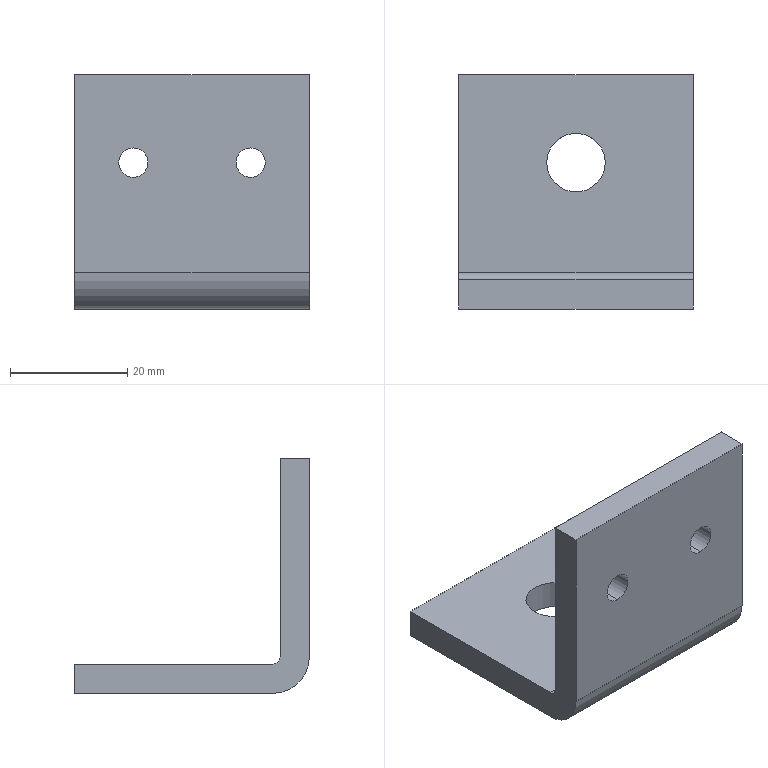Part | SolidWorks | features ICE 2, Extrusion 1 | 1 solid | 16 faces | box 40 x 40 x 40 mm | volume 14089 mm3 | cylinder 8 | plane 8 | commonest cylinder face diameters 5 x4 10 x2 2.5 x1 12.5 x1
STEP:
#1=CARTESIAN_POINT('',(-0.3937,-0.5659,0.421));
#2=VERTEX_POINT('',#1);
#3=CARTESIAN_POINT('',(-0.3937,-0.5659,0.2242));
#4=VERTEX_POINT('',#3);
#5=CARTESIAN_POINT('',(-0.3937,-0.5659,0.3226));
#6=DIRECTION('',(0.,-1.,0.));
#7=DIRECTION('',(0.,0.,-1.));
#8=AXIS2_PLACEMENT_3D('',#5,#6,#7);
#9=CIRCLE('',#8,0.09843);
#10=EDGE_CURVE('',#2,#4,#9,.T.);
#11=ORIENTED_EDGE('',*,*,#10,.T.);
#12=CARTESIAN_POINT('',(-0.3937,-0.3691,0.2242));
#13=VERTEX_POINT('',#12);
#14=CARTESIAN_POINT('',(-0.3937,-1.944,0.2242));
#15=DIRECTION('',(0.,1.,0.));
#16=VECTOR('',#15,39.37);
#17=LINE('',#14,#16);
#18=EDGE_CURVE('',#4,#13,#17,.T.);
#19=ORIENTED_EDGE('',*,*,#18,.T.);
#20=CARTESIAN_POINT('',(-0.3937,-0.3691,0.421));
#21=VERTEX_POINT('',#20);
#22=CARTESIAN_POINT('',(-0.3937,-0.3691,0.3226));
#23=DIRECTION('',(0.,1.,0.));
#24=DIRECTION('',(0.,0.,1.));
#25=AXIS2_PLACEMENT_3D('',#22,#23,#24);
#26=CIRCLE('',#25,0.09843);
#27=EDGE_CURVE('',#13,#21,#26,.T.);
#28=ORIENTED_EDGE('',*,*,#27,.T.);
#29=CARTESIAN_POINT('',(-0.3937,-1.944,0.421));
#30=DIRECTION('',(0.,1.,0.));
#31=VECTOR('',#30,39.37);
#32=LINE('',#29,#31);
#33=EDGE_CURVE('',#2,#21,#32,.T.);
#34=ORIENTED_EDGE('',*,*,#33,.F.);
#35=EDGE_LOOP('',(#11,#19,#28,#34));
#36=FACE_OUTER_BOUND('',#35,.T.);
#37=CARTESIAN_POINT('',(-0.3937,-1.944,0.3226));
#38=DIRECTION('',(0.,1.,0.));
#39=DIRECTION('',(0.,0.,1.));
#40=AXIS2_PLACEMENT_3D('',#37,#38,#39);
#41=CYLINDRICAL_SURFACE('',#40,0.09843);
#42=ADVANCED_FACE('',(#36),#41,.F.);
#43=CARTESIAN_POINT('',(-1.181,-0.5659,0.421));
#44=VERTEX_POINT('',#43);
#45=CARTESIAN_POINT('',(-1.181,-0.5659,0.2242));
#46=VERTEX_POINT('',#45);
#47=CARTESIAN_POINT('',(-1.181,-0.5659,0.3226));
#48=DIRECTION('',(0.,-1.,0.));
#49=DIRECTION('',(0.,0.,-1.));
#50=AXIS2_PLACEMENT_3D('',#47,#48,#49);
#51=CIRCLE('',#50,0.09843);
#52=EDGE_CURVE('',#44,#46,#51,.T.);
#53=ORIENTED_EDGE('',*,*,#52,.T.);
#54=CARTESIAN_POINT('',(-1.181,-0.3691,0.2242));
#55=VERTEX_POINT('',#54);
#56=CARTESIAN_POINT('',(-1.181,-1.944,0.2242));
#57=DIRECTION('',(0.,1.,0.));
#58=VECTOR('',#57,39.37);
#59=LINE('',#56,#58);
#60=EDGE_CURVE('',#46,#55,#59,.T.);
#61=ORIENTED_EDGE('',*,*,#60,.T.);
#62=CARTESIAN_POINT('',(-1.181,-0.3691,0.421));
#63=VERTEX_POINT('',#62);
#64=CARTESIAN_POINT('',(-1.181,-0.3691,0.3226));
#65=DIRECTION('',(0.,1.,0.));
#66=DIRECTION('',(0.,0.,1.));
#67=AXIS2_PLACEMENT_3D('',#64,#65,#66);
#68=CIRCLE('',#67,0.09843);
#69=EDGE_CURVE('',#55,#63,#68,.T.);
#70=ORIENTED_EDGE('',*,*,#69,.T.);
#71=CARTESIAN_POINT('',(-1.181,-1.944,0.421));
#72=DIRECTION('',(0.,1.,0.));
#73=VECTOR('',#72,39.37);
#74=LINE('',#71,#73);
#75=EDGE_CURVE('',#44,#63,#74,.T.);
#76=ORIENTED_EDGE('',*,*,#75,.F.);
#77=EDGE_LOOP('',(#53,#61,#70,#76));
#78=FACE_OUTER_BOUND('',#77,.T.);
#79=CARTESIAN_POINT('',(-1.181,-1.944,0.3226));
#80=DIRECTION('',(0.,1.,0.));
#81=DIRECTION('',(0.,0.,1.));
#82=AXIS2_PLACEMENT_3D('',#79,#80,#81);
#83=CYLINDRICAL_SURFACE('',#82,0.09843);
#84=ADVANCED_FACE('',(#78),#83,.F.);
#85=CARTESIAN_POINT('',(-0.5906,0.4183,-0.6616));
#86=VERTEX_POINT('',#85);
#87=CARTESIAN_POINT('',(-0.9843,0.4183,-0.6616));
#88=VERTEX_POINT('',#87);
#89=CARTESIAN_POINT('',(-0.7874,0.4183,-0.6616));
#90=DIRECTION('',(0.,0.,-1.));
#91=DIRECTION('',(-1.,0.,0.));
#92=AXIS2_PLACEMENT_3D('',#89,#90,#91);
#93=CIRCLE('',#92,0.1969);
#94=EDGE_CURVE('',#86,#88,#93,.T.);
#95=ORIENTED_EDGE('',*,*,#94,.T.);
#96=CARTESIAN_POINT('',(-0.9843,0.4183,-0.4648));
#97=VERTEX_POINT('',#96);
#98=CARTESIAN_POINT('',(-0.9843,0.4183,-2.04));
#99=DIRECTION('',(0.,0.,1.));
#100=VECTOR('',#99,39.37);
#101=LINE('',#98,#100);
#102=EDGE_CURVE('',#88,#97,#101,.T.);
#103=ORIENTED_EDGE('',*,*,#102,.T.);
#104=CARTESIAN_POINT('',(-0.5906,0.4183,-0.4648));
#105=VERTEX_POINT('',#104);
#106=CARTESIAN_POINT('',(-0.7874,0.4183,-0.4648));
#107=DIRECTION('',(0.,0.,1.));
#108=DIRECTION('',(1.,0.,0.));
#109=AXIS2_PLACEMENT_3D('',#106,#107,#108);
#110=CIRCLE('',#109,0.1969);
#111=EDGE_CURVE('',#97,#105,#110,.T.);
#112=ORIENTED_EDGE('',*,*,#111,.T.);
#113=CARTESIAN_POINT('',(-0.5906,0.4183,-2.04));
#114=DIRECTION('',(0.,0.,1.));
#115=VECTOR('',#114,39.37);
#116=LINE('',#113,#115);
#117=EDGE_CURVE('',#86,#105,#116,.T.);
#118=ORIENTED_EDGE('',*,*,#117,.F.);
#119=EDGE_LOOP('',(#95,#103,#112,#118));
#120=FACE_OUTER_BOUND('',#119,.T.);
#121=CARTESIAN_POINT('',(-0.7874,0.4183,-2.04));
#122=DIRECTION('',(0.,0.,1.));
#123=DIRECTION('',(1.,0.,0.));
#124=AXIS2_PLACEMENT_3D('',#121,#122,#123);
#125=CYLINDRICAL_SURFACE('',#124,0.1969);
#126=ADVANCED_FACE('',(#120),#125,.F.);
#127=CARTESIAN_POINT('',(0.,1.009,-0.6616));
#128=VERTEX_POINT('',#127);
#129=CARTESIAN_POINT('',(0.,1.009,-0.4648));
#130=VERTEX_POINT('',#129);
#131=CARTESIAN_POINT('',(0.,1.009,-0.6616));
#132=DIRECTION('',(0.,0.,1.));
#133=VECTOR('',#132,39.37);
#134=LINE('',#131,#133);
#135=EDGE_CURVE('',#128,#130,#134,.T.);
#136=ORIENTED_EDGE('',*,*,#135,.F.);
#137=CARTESIAN_POINT('',(-1.575,1.009,-0.6616));
#138=VERTEX_POINT('',#137);
#139=CARTESIAN_POINT('',(-1.575,1.009,-0.6616));
#140=DIRECTION('',(1.,0.,0.));
#141=VECTOR('',#140,39.37);
#142=LINE('',#139,#141);
#143=EDGE_CURVE('',#138,#128,#142,.T.);
#144=ORIENTED_EDGE('',*,*,#143,.F.);
#145=CARTESIAN_POINT('',(-1.575,1.009,-0.4648));
#146=VERTEX_POINT('',#145);
#147=CARTESIAN_POINT('',(-1.575,1.009,-0.6616));
#148=DIRECTION('',(0.,0.,1.));
#149=VECTOR('',#148,39.37);
#150=LINE('',#147,#149);
#151=EDGE_CURVE('',#138,#146,#150,.T.);
#152=ORIENTED_EDGE('',*,*,#151,.T.);
#153=CARTESIAN_POINT('',(-1.575,1.009,-0.4648));
#154=DIRECTION('',(1.,0.,0.));
#155=VECTOR('',#154,39.37);
#156=LINE('',#153,#155);
#157=EDGE_CURVE('',#146,#130,#156,.T.);
#158=ORIENTED_EDGE('',*,*,#157,.T.);
#159=EDGE_LOOP('',(#136,#144,#152,#158));
#160=FACE_OUTER_BOUND('',#159,.T.);
#161=CARTESIAN_POINT('',(-1.575,1.009,-0.6616));
#162=DIRECTION('',(0.,1.,0.));
#163=DIRECTION('',(0.,0.,1.));
#164=AXIS2_PLACEMENT_3D('',#161,#162,#163);
#165=PLANE('',#164);
#166=ADVANCED_FACE('',(#160),#165,.T.);
#167=ORIENTED_EDGE('',*,*,#94,.F.);
#168=CARTESIAN_POINT('',(-0.7874,0.4183,-0.6616));
#169=DIRECTION('',(0.,0.,-1.));
#170=DIRECTION('',(-1.,0.,0.));
#171=AXIS2_PLACEMENT_3D('',#168,#169,#170);
#172=CIRCLE('',#171,0.1969);
#173=EDGE_CURVE('',#88,#86,#172,.T.);
#174=ORIENTED_EDGE('',*,*,#173,.F.);
#175=EDGE_LOOP('',(#167,#174));
#176=FACE_BOUND('',#175,.T.);
#177=CARTESIAN_POINT('',(0.,-0.3199,-0.6616));
#178=VERTEX_POINT('',#177);
#179=CARTESIAN_POINT('',(0.,-0.3199,-0.6616));
#180=DIRECTION('',(0.,1.,0.));
#181=VECTOR('',#180,39.37);
#182=LINE('',#179,#181);
#183=EDGE_CURVE('',#178,#128,#182,.T.);
#184=ORIENTED_EDGE('',*,*,#183,.F.);
#185=CARTESIAN_POINT('',(-1.575,-0.3199,-0.6616));
#186=VERTEX_POINT('',#185);
#187=CARTESIAN_POINT('',(-1.575,-0.3199,-0.6616));
#188=DIRECTION('',(1.,0.,0.));
#189=VECTOR('',#188,39.37);
#190=LINE('',#187,#189);
#191=EDGE_CURVE('',#186,#178,#190,.T.);
#192=ORIENTED_EDGE('',*,*,#191,.F.);
#193=CARTESIAN_POINT('',(-1.575,-0.3199,-0.6616));
#194=DIRECTION('',(0.,1.,0.));
#195=VECTOR('',#194,39.37);
#196=LINE('',#193,#195);
#197=EDGE_CURVE('',#186,#138,#196,.T.);
#198=ORIENTED_EDGE('',*,*,#197,.T.);
#199=ORIENTED_EDGE('',*,*,#143,.T.);
#200=EDGE_LOOP('',(#184,#192,#198,#199));
#201=FACE_OUTER_BOUND('',#200,.T.);
#202=CARTESIAN_POINT('',(-1.575,-0.3199,-0.6616));
#203=DIRECTION('',(0.,0.,-1.));
#204=DIRECTION('',(-1.,0.,0.));
#205=AXIS2_PLACEMENT_3D('',#202,#203,#204);
#206=PLANE('',#205);
#207=ADVANCED_FACE('',(#176,#201),#206,.T.);
#208=CARTESIAN_POINT('',(0.,-0.5659,-0.4156));
#209=VERTEX_POINT('',#208);
#210=CARTESIAN_POINT('',(0.,-0.3199,-0.4156));
#211=DIRECTION('',(1.,0.,0.));
#212=DIRECTION('',(0.,0.,1.));
#213=AXIS2_PLACEMENT_3D('',#210,#211,#212);
#214=CIRCLE('',#213,0.2461);
#215=EDGE_CURVE('',#209,#178,#214,.T.);
#216=ORIENTED_EDGE('',*,*,#215,.F.);
#217=CARTESIAN_POINT('',(-1.575,-0.5659,-0.4156));
#218=VERTEX_POINT('',#217);
#219=CARTESIAN_POINT('',(-1.575,-0.5659,-0.4156));
#220=DIRECTION('',(1.,0.,0.));
#221=VECTOR('',#220,39.37);
#222=LINE('',#219,#221);
#223=EDGE_CURVE('',#218,#209,#222,.T.);
#224=ORIENTED_EDGE('',*,*,#223,.F.);
#225=CARTESIAN_POINT('',(-1.575,-0.3199,-0.4156));
#226=DIRECTION('',(1.,0.,0.));
#227=DIRECTION('',(0.,0.,1.));
#228=AXIS2_PLACEMENT_3D('',#225,#226,#227);
#229=CIRCLE('',#228,0.2461);
#230=EDGE_CURVE('',#218,#186,#229,.T.);
#231=ORIENTED_EDGE('',*,*,#230,.T.);
#232=ORIENTED_EDGE('',*,*,#191,.T.);
#233=EDGE_LOOP('',(#216,#224,#231,#232));
#234=FACE_OUTER_BOUND('',#233,.T.);
#235=CARTESIAN_POINT('',(-1.575,-0.3199,-0.4156));
#236=DIRECTION('',(1.,0.,0.));
#237=DIRECTION('',(0.,0.,-1.));
#238=AXIS2_PLACEMENT_3D('',#235,#236,#237);
#239=CYLINDRICAL_SURFACE('',#238,0.2461);
#240=ADVANCED_FACE('',(#234),#239,.T.);
#241=ORIENTED_EDGE('',*,*,#10,.F.);
#242=CARTESIAN_POINT('',(-0.3937,-0.5659,0.3226));
#243=DIRECTION('',(0.,-1.,0.));
#244=DIRECTION('',(0.,0.,-1.));
#245=AXIS2_PLACEMENT_3D('',#242,#243,#244);
#246=CIRCLE('',#245,0.09843);
#247=EDGE_CURVE('',#4,#2,#246,.T.);
#248=ORIENTED_EDGE('',*,*,#247,.F.);
#249=EDGE_LOOP('',(#241,#248));
#250=FACE_BOUND('',#249,.T.);
#251=ORIENTED_EDGE('',*,*,#52,.F.);
#252=CARTESIAN_POINT('',(-1.181,-0.5659,0.3226));
#253=DIRECTION('',(0.,-1.,0.));
#254=DIRECTION('',(0.,0.,-1.));
#255=AXIS2_PLACEMENT_3D('',#252,#253,#254);
#256=CIRCLE('',#255,0.09843);
#257=EDGE_CURVE('',#46,#44,#256,.T.);
#258=ORIENTED_EDGE('',*,*,#257,.F.);
#259=EDGE_LOOP('',(#251,#258));
#260=FACE_BOUND('',#259,.T.);
#261=CARTESIAN_POINT('',(0.,-0.5659,0.9132));
#262=VERTEX_POINT('',#261);
#263=CARTESIAN_POINT('',(0.,-0.5659,0.9132));
#264=DIRECTION('',(0.,0.,-1.));
#265=VECTOR('',#264,39.37);
#266=LINE('',#263,#265);
#267=EDGE_CURVE('',#262,#209,#266,.T.);
#268=ORIENTED_EDGE('',*,*,#267,.F.);
#269=CARTESIAN_POINT('',(-1.575,-0.5659,0.9132));
#270=VERTEX_POINT('',#269);
#271=CARTESIAN_POINT('',(-1.575,-0.5659,0.9132));
#272=DIRECTION('',(1.,0.,0.));
#273=VECTOR('',#272,39.37);
#274=LINE('',#271,#273);
#275=EDGE_CURVE('',#270,#262,#274,.T.);
#276=ORIENTED_EDGE('',*,*,#275,.F.);
#277=CARTESIAN_POINT('',(-1.575,-0.5659,0.9132));
#278=DIRECTION('',(0.,0.,-1.));
#279=VECTOR('',#278,39.37);
#280=LINE('',#277,#279);
#281=EDGE_CURVE('',#270,#218,#280,.T.);
#282=ORIENTED_EDGE('',*,*,#281,.T.);
#283=ORIENTED_EDGE('',*,*,#223,.T.);
#284=EDGE_LOOP('',(#268,#276,#282,#283));
#285=FACE_OUTER_BOUND('',#284,.T.);
#286=CARTESIAN_POINT('',(-1.575,-0.5659,0.9132));
#287=DIRECTION('',(0.,-1.,0.));
#288=DIRECTION('',(0.,0.,-1.));
#289=AXIS2_PLACEMENT_3D('',#286,#287,#288);
#290=PLANE('',#289);
#291=ADVANCED_FACE('',(#250,#260,#285),#290,.T.);
#292=CARTESIAN_POINT('',(0.,-0.3691,0.9132));
#293=VERTEX_POINT('',#292);
#294=CARTESIAN_POINT('',(0.,-0.3691,0.9132));
#295=DIRECTION('',(0.,-1.,0.));
#296=VECTOR('',#295,39.37);
#297=LINE('',#294,#296);
#298=EDGE_CURVE('',#293,#262,#297,.T.);
#299=ORIENTED_EDGE('',*,*,#298,.F.);
#300=CARTESIAN_POINT('',(-1.575,-0.3691,0.9132));
#301=VERTEX_POINT('',#300);
#302=CARTESIAN_POINT('',(-1.575,-0.3691,0.9132));
#303=DIRECTION('',(1.,0.,0.));
#304=VECTOR('',#303,39.37);
#305=LINE('',#302,#304);
#306=EDGE_CURVE('',#301,#293,#305,.T.);
#307=ORIENTED_EDGE('',*,*,#306,.F.);
#308=CARTESIAN_POINT('',(-1.575,-0.3691,0.9132));
#309=DIRECTION('',(0.,-1.,0.));
#310=VECTOR('',#309,39.37);
#311=LINE('',#308,#310);
#312=EDGE_CURVE('',#301,#270,#311,.T.);
#313=ORIENTED_EDGE('',*,*,#312,.T.);
#314=ORIENTED_EDGE('',*,*,#275,.T.);
#315=EDGE_LOOP('',(#299,#307,#313,#314));
#316=FACE_OUTER_BOUND('',#315,.T.);
#317=CARTESIAN_POINT('',(-1.575,-0.3691,0.9132));
#318=DIRECTION('',(0.,0.,1.));
#319=DIRECTION('',(1.,0.,0.));
#320=AXIS2_PLACEMENT_3D('',#317,#318,#319);
#321=PLANE('',#320);
#322=ADVANCED_FACE('',(#316),#321,.T.);
#323=CARTESIAN_POINT('',(-0.3937,-0.3691,0.3226));
#324=DIRECTION('',(0.,1.,0.));
#325=DIRECTION('',(0.,0.,1.));
#326=AXIS2_PLACEMENT_3D('',#323,#324,#325);
#327=CIRCLE('',#326,0.09843);
#328=EDGE_CURVE('',#21,#13,#327,.T.);
#329=ORIENTED_EDGE('',*,*,#328,.F.);
#330=ORIENTED_EDGE('',*,*,#27,.F.);
#331=EDGE_LOOP('',(#329,#330));
#332=FACE_BOUND('',#331,.T.);
#333=CARTESIAN_POINT('',(-1.181,-0.3691,0.3226));
#334=DIRECTION('',(0.,1.,0.));
#335=DIRECTION('',(0.,0.,1.));
#336=AXIS2_PLACEMENT_3D('',#333,#334,#335);
#337=CIRCLE('',#336,0.09843);
#338=EDGE_CURVE('',#63,#55,#337,.T.);
#339=ORIENTED_EDGE('',*,*,#338,.F.);
#340=ORIENTED_EDGE('',*,*,#69,.F.);
#341=EDGE_LOOP('',(#339,#340));
#342=FACE_BOUND('',#341,.T.);
#343=CARTESIAN_POINT('',(0.,-0.3691,-0.4156));
#344=VERTEX_POINT('',#343);
#345=CARTESIAN_POINT('',(0.,-0.3691,-0.4156));
#346=DIRECTION('',(0.,0.,1.));
#347=VECTOR('',#346,39.37);
#348=LINE('',#345,#347);
#349=EDGE_CURVE('',#344,#293,#348,.T.);
#350=ORIENTED_EDGE('',*,*,#349,.F.);
#351=CARTESIAN_POINT('',(-1.575,-0.3691,-0.4156));
#352=VERTEX_POINT('',#351);
#353=CARTESIAN_POINT('',(-1.575,-0.3691,-0.4156));
#354=DIRECTION('',(1.,0.,0.));
#355=VECTOR('',#354,39.37);
#356=LINE('',#353,#355);
#357=EDGE_CURVE('',#352,#344,#356,.T.);
#358=ORIENTED_EDGE('',*,*,#357,.F.);
#359=CARTESIAN_POINT('',(-1.575,-0.3691,-0.4156));
#360=DIRECTION('',(0.,0.,1.));
#361=VECTOR('',#360,39.37);
#362=LINE('',#359,#361);
#363=EDGE_CURVE('',#352,#301,#362,.T.);
#364=ORIENTED_EDGE('',*,*,#363,.T.);
#365=ORIENTED_EDGE('',*,*,#306,.T.);
#366=EDGE_LOOP('',(#350,#358,#364,#365));
#367=FACE_OUTER_BOUND('',#366,.T.);
#368=CARTESIAN_POINT('',(-1.575,-0.3691,-0.4156));
#369=DIRECTION('',(0.,1.,0.));
#370=DIRECTION('',(0.,0.,1.));
#371=AXIS2_PLACEMENT_3D('',#368,#369,#370);
#372=PLANE('',#371);
#373=ADVANCED_FACE('',(#332,#342,#367),#372,.T.);
#374=CARTESIAN_POINT('',(0.,-0.3199,-0.4648));
#375=VERTEX_POINT('',#374);
#376=CARTESIAN_POINT('',(0.,-0.3199,-0.4156));
#377=DIRECTION('',(-1.,0.,0.));
#378=DIRECTION('',(0.,0.,1.));
#379=AXIS2_PLACEMENT_3D('',#376,#377,#378);
#380=CIRCLE('',#379,0.04921);
#381=EDGE_CURVE('',#375,#344,#380,.T.);
#382=ORIENTED_EDGE('',*,*,#381,.F.);
#383=CARTESIAN_POINT('',(-1.575,-0.3199,-0.4648));
#384=VERTEX_POINT('',#383);
#385=CARTESIAN_POINT('',(-1.575,-0.3199,-0.4648));
#386=DIRECTION('',(1.,0.,0.));
#387=VECTOR('',#386,39.37);
#388=LINE('',#385,#387);
#389=EDGE_CURVE('',#384,#375,#388,.T.);
#390=ORIENTED_EDGE('',*,*,#389,.F.);
#391=CARTESIAN_POINT('',(-1.575,-0.3199,-0.4156));
#392=DIRECTION('',(-1.,0.,0.));
#393=DIRECTION('',(0.,0.,1.));
#394=AXIS2_PLACEMENT_3D('',#391,#392,#393);
#395=CIRCLE('',#394,0.04921);
#396=EDGE_CURVE('',#384,#352,#395,.T.);
#397=ORIENTED_EDGE('',*,*,#396,.T.);
#398=ORIENTED_EDGE('',*,*,#357,.T.);
#399=EDGE_LOOP('',(#382,#390,#397,#398));
#400=FACE_OUTER_BOUND('',#399,.T.);
#401=CARTESIAN_POINT('',(-1.575,-0.3199,-0.4156));
#402=DIRECTION('',(1.,0.,0.));
#403=DIRECTION('',(0.,0.,-1.));
#404=AXIS2_PLACEMENT_3D('',#401,#402,#403);
#405=CYLINDRICAL_SURFACE('',#404,0.04921);
#406=ADVANCED_FACE('',(#400),#405,.F.);
#407=CARTESIAN_POINT('',(-0.7874,0.4183,-0.4648));
#408=DIRECTION('',(0.,0.,1.));
#409=DIRECTION('',(1.,0.,0.));
#410=AXIS2_PLACEMENT_3D('',#407,#408,#409);
#411=CIRCLE('',#410,0.1969);
#412=EDGE_CURVE('',#105,#97,#411,.T.);
#413=ORIENTED_EDGE('',*,*,#412,.F.);
#414=ORIENTED_EDGE('',*,*,#111,.F.);
#415=EDGE_LOOP('',(#413,#414));
#416=FACE_BOUND('',#415,.T.);
#417=CARTESIAN_POINT('',(0.,1.009,-0.4648));
#418=DIRECTION('',(0.,-1.,0.));
#419=VECTOR('',#418,39.37);
#420=LINE('',#417,#419);
#421=EDGE_CURVE('',#130,#375,#420,.T.);
#422=ORIENTED_EDGE('',*,*,#421,.F.);
#423=ORIENTED_EDGE('',*,*,#157,.F.);
#424=CARTESIAN_POINT('',(-1.575,1.009,-0.4648));
#425=DIRECTION('',(0.,-1.,0.));
#426=VECTOR('',#425,39.37);
#427=LINE('',#424,#426);
#428=EDGE_CURVE('',#146,#384,#427,.T.);
#429=ORIENTED_EDGE('',*,*,#428,.T.);
#430=ORIENTED_EDGE('',*,*,#389,.T.);
#431=EDGE_LOOP('',(#422,#423,#429,#430));
#432=FACE_OUTER_BOUND('',#431,.T.);
#433=CARTESIAN_POINT('',(-1.575,1.009,-0.4648));
#434=DIRECTION('',(0.,0.,1.));
#435=DIRECTION('',(1.,0.,0.));
#436=AXIS2_PLACEMENT_3D('',#433,#434,#435);
#437=PLANE('',#436);
#438=ADVANCED_FACE('',(#416,#432),#437,.T.);
#439=ORIENTED_EDGE('',*,*,#151,.F.);
#440=ORIENTED_EDGE('',*,*,#197,.F.);
#441=ORIENTED_EDGE('',*,*,#230,.F.);
#442=ORIENTED_EDGE('',*,*,#281,.F.);
#443=ORIENTED_EDGE('',*,*,#312,.F.);
#444=ORIENTED_EDGE('',*,*,#363,.F.);
#445=ORIENTED_EDGE('',*,*,#396,.F.);
#446=ORIENTED_EDGE('',*,*,#428,.F.);
#447=EDGE_LOOP('',(#439,#440,#441,#442,#443,#444,#445,#446));
#448=FACE_OUTER_BOUND('',#447,.T.);
#449=CARTESIAN_POINT('',(-1.575,-0.3199,-0.4156));
#450=DIRECTION('',(-1.,0.,0.));
#451=DIRECTION('',(0.,0.,1.));
#452=AXIS2_PLACEMENT_3D('',#449,#450,#451);
#453=PLANE('',#452);
#454=ADVANCED_FACE('',(#448),#453,.T.);
#455=ORIENTED_EDGE('',*,*,#135,.T.);
#456=ORIENTED_EDGE('',*,*,#421,.T.);
#457=ORIENTED_EDGE('',*,*,#381,.T.);
#458=ORIENTED_EDGE('',*,*,#349,.T.);
#459=ORIENTED_EDGE('',*,*,#298,.T.);
#460=ORIENTED_EDGE('',*,*,#267,.T.);
#461=ORIENTED_EDGE('',*,*,#215,.T.);
#462=ORIENTED_EDGE('',*,*,#183,.T.);
#463=EDGE_LOOP('',(#455,#456,#457,#458,#459,#460,#461,#462));
#464=FACE_OUTER_BOUND('',#463,.T.);
#465=CARTESIAN_POINT('',(0.,-0.3199,-0.4156));
#466=DIRECTION('',(-1.,0.,0.));
#467=DIRECTION('',(0.,0.,1.));
#468=AXIS2_PLACEMENT_3D('',#465,#466,#467);
#469=PLANE('',#468);
#470=ADVANCED_FACE('',(#464),#469,.F.);
#471=ORIENTED_EDGE('',*,*,#102,.F.);
#472=ORIENTED_EDGE('',*,*,#173,.T.);
#473=ORIENTED_EDGE('',*,*,#117,.T.);
#474=ORIENTED_EDGE('',*,*,#412,.T.);
#475=EDGE_LOOP('',(#471,#472,#473,#474));
#476=FACE_OUTER_BOUND('',#475,.T.);
#477=CARTESIAN_POINT('',(-0.7874,0.4183,-2.04));
#478=DIRECTION('',(0.,0.,1.));
#479=DIRECTION('',(1.,0.,0.));
#480=AXIS2_PLACEMENT_3D('',#477,#478,#479);
#481=CYLINDRICAL_SURFACE('',#480,0.1969);
#482=ADVANCED_FACE('',(#476),#481,.F.);
#483=ORIENTED_EDGE('',*,*,#60,.F.);
#484=ORIENTED_EDGE('',*,*,#257,.T.);
#485=ORIENTED_EDGE('',*,*,#75,.T.);
#486=ORIENTED_EDGE('',*,*,#338,.T.);
#487=EDGE_LOOP('',(#483,#484,#485,#486));
#488=FACE_OUTER_BOUND('',#487,.T.);
#489=CARTESIAN_POINT('',(-1.181,-1.944,0.3226));
#490=DIRECTION('',(0.,1.,0.));
#491=DIRECTION('',(0.,0.,1.));
#492=AXIS2_PLACEMENT_3D('',#489,#490,#491);
#493=CYLINDRICAL_SURFACE('',#492,0.09843);
#494=ADVANCED_FACE('',(#488),#493,.F.);
#495=ORIENTED_EDGE('',*,*,#18,.F.);
#496=ORIENTED_EDGE('',*,*,#247,.T.);
#497=ORIENTED_EDGE('',*,*,#33,.T.);
#498=ORIENTED_EDGE('',*,*,#328,.T.);
#499=EDGE_LOOP('',(#495,#496,#497,#498));
#500=FACE_OUTER_BOUND('',#499,.T.);
#501=CARTESIAN_POINT('',(-0.3937,-1.944,0.3226));
#502=DIRECTION('',(0.,1.,0.));
#503=DIRECTION('',(0.,0.,1.));
#504=AXIS2_PLACEMENT_3D('',#501,#502,#503);
#505=CYLINDRICAL_SURFACE('',#504,0.09843);
#506=ADVANCED_FACE('',(#500),#505,.F.);
#507=CLOSED_SHELL('',(#42,#84,#126,#166,#207,#240,#291,#322,#373,#406,#438,#454,#470,#482,#494,#506));
#508=MANIFOLD_SOLID_BREP('',#507);
#509=CARTESIAN_POINT('',(0.,0.,0.));
#510=DIRECTION('',(0.,0.,1.));
#511=DIRECTION('',(1.,0.,0.));
#512=AXIS2_PLACEMENT_3D('',#509,#510,#511);
#513=(LENGTH_UNIT()NAMED_UNIT(*)SI_UNIT($,.METRE.));
#514=LENGTH_MEASURE_WITH_UNIT(LENGTH_MEASURE(0.0254),#513);
#515=DIMENSIONAL_EXPONENTS(1.,0.,0.,0.,0.,0.,0.);
#516=(CONVERSION_BASED_UNIT('INCH',#514)LENGTH_UNIT()NAMED_UNIT(#515));
#517=UNCERTAINTY_MEASURE_WITH_UNIT(LENGTH_MEASURE(0.00001),#516,'','');
#518=(NAMED_UNIT(*)PLANE_ANGLE_UNIT()SI_UNIT($,.RADIAN.));
#519=(NAMED_UNIT(*)SI_UNIT($,.STERADIAN.)SOLID_ANGLE_UNIT());
#520=(GEOMETRIC_REPRESENTATION_CONTEXT(3)GLOBAL_UNCERTAINTY_ASSIGNED_CONTEXT((#517))GLOBAL_UNIT_ASSIGNED_CONTEXT((#516,#518,#519))REPRESENTATION_CONTEXT('',''));
#521=ADVANCED_BREP_SHAPE_REPRESENTATION('',(#508,#512),#520);